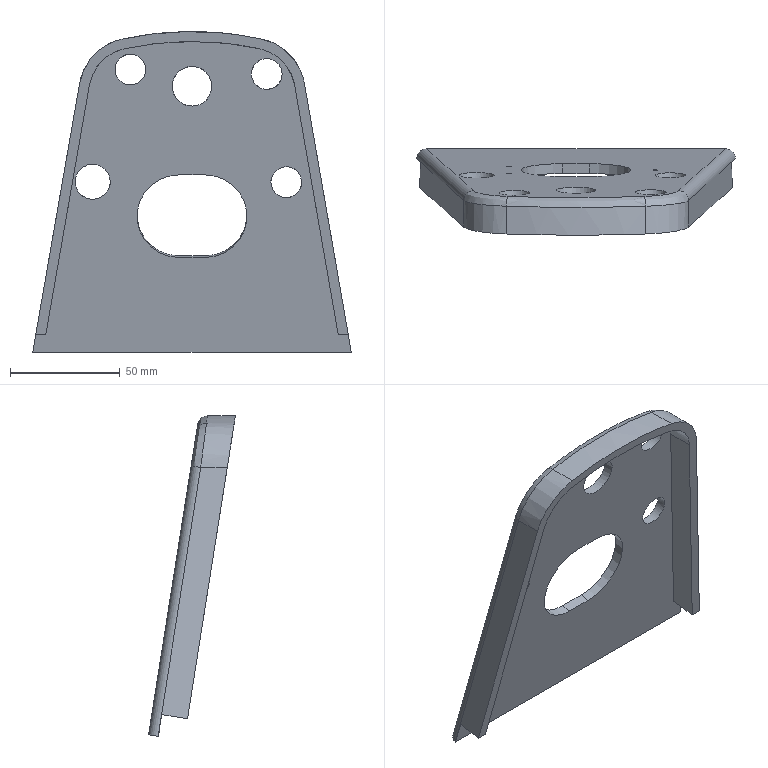Part | STEP file | 1-56.10 | 1 solid | 36 faces | box 144.937 x 39.504 x 145.902 mm | volume 83548 mm3 | cylinder 18 | plane 15 | spline 3 | commonest cylinder face diameters 2 x3 14 x3 9 x2 38 x2 41 x2 50 x2